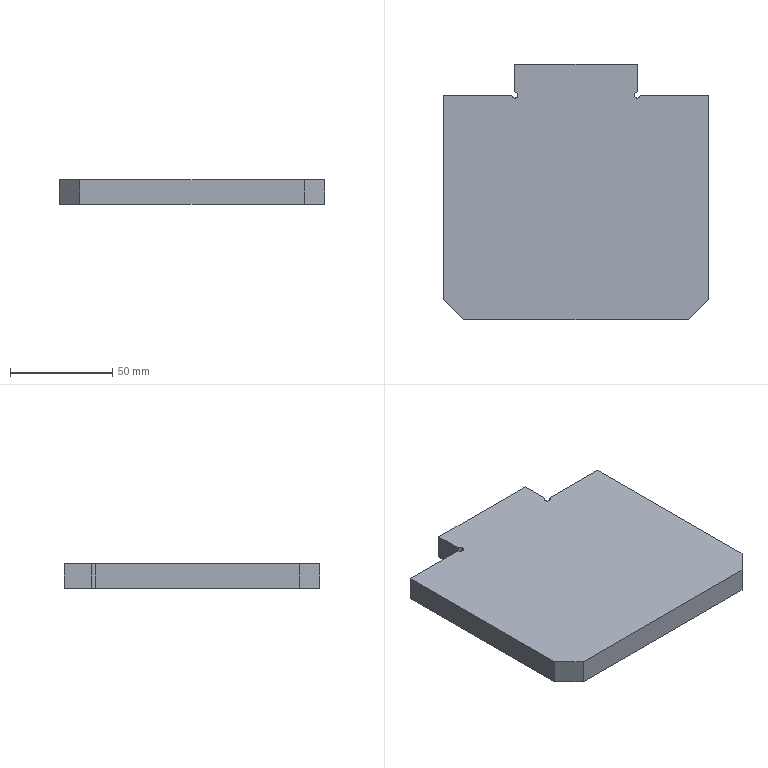Part | SolidWorks | features BaseBody 1 | 1 solid | 15 faces | box 130 x 125 x 12 mm | volume 181073 mm3 | plane 12 | cylinder 3 | commonest cylinder face diameters 3 x3
STEP:
#1=CARTESIAN_POINT('',(-28.5,55.,-6.));
#2=VERTEX_POINT('',#1);
#3=CARTESIAN_POINT('',(-30.,56.5,-6.));
#4=VERTEX_POINT('',#3);
#5=CARTESIAN_POINT('',(-30.,55.,-6.));
#6=DIRECTION('',(0.,0.,1.));
#7=DIRECTION('',(1.,0.,0.));
#8=AXIS2_PLACEMENT_3D('',#5,#6,#7);
#9=CIRCLE('',#8,1.5);
#10=EDGE_CURVE('',#2,#4,#9,.T.);
#11=ORIENTED_EDGE('',*,*,#10,.F.);
#12=CARTESIAN_POINT('',(-28.5,55.,6.));
#13=VERTEX_POINT('',#12);
#14=CARTESIAN_POINT('',(-28.5,55.,-7.));
#15=DIRECTION('',(0.,0.,1.));
#16=VECTOR('',#15,1000.);
#17=LINE('',#14,#16);
#18=EDGE_CURVE('',#2,#13,#17,.T.);
#19=ORIENTED_EDGE('',*,*,#18,.T.);
#20=CARTESIAN_POINT('',(-30.,56.5,6.));
#21=VERTEX_POINT('',#20);
#22=CARTESIAN_POINT('',(-30.,55.,6.));
#23=DIRECTION('',(0.,0.,1.));
#24=DIRECTION('',(1.,0.,0.));
#25=AXIS2_PLACEMENT_3D('',#22,#23,#24);
#26=CIRCLE('',#25,1.5);
#27=EDGE_CURVE('',#13,#21,#26,.T.);
#28=ORIENTED_EDGE('',*,*,#27,.T.);
#29=CARTESIAN_POINT('',(-30.,56.5,-7.));
#30=DIRECTION('',(0.,0.,1.));
#31=VECTOR('',#30,1000.);
#32=LINE('',#29,#31);
#33=EDGE_CURVE('',#4,#21,#32,.T.);
#34=ORIENTED_EDGE('',*,*,#33,.F.);
#35=EDGE_LOOP('',(#11,#19,#28,#34));
#36=FACE_OUTER_BOUND('',#35,.T.);
#37=CARTESIAN_POINT('',(-30.,55.,-7.));
#38=DIRECTION('',(0.,0.,1.));
#39=DIRECTION('',(1.,0.,0.));
#40=AXIS2_PLACEMENT_3D('',#37,#38,#39);
#41=CYLINDRICAL_SURFACE('',#40,1.5);
#42=ADVANCED_FACE('',(#36),#41,.F.);
#43=CARTESIAN_POINT('',(65.,55.,-6.));
#44=VERTEX_POINT('',#43);
#45=CARTESIAN_POINT('',(31.5,55.,-6.));
#46=VERTEX_POINT('',#45);
#47=CARTESIAN_POINT('',(-65.,55.,-6.));
#48=DIRECTION('',(-1.,0.,0.));
#49=VECTOR('',#48,1000.);
#50=LINE('',#47,#49);
#51=EDGE_CURVE('',#44,#46,#50,.T.);
#52=ORIENTED_EDGE('',*,*,#51,.T.);
#53=CARTESIAN_POINT('',(31.5,55.,6.));
#54=VERTEX_POINT('',#53);
#55=CARTESIAN_POINT('',(31.5,55.,-7.));
#56=DIRECTION('',(0.,0.,1.));
#57=VECTOR('',#56,1000.);
#58=LINE('',#55,#57);
#59=EDGE_CURVE('',#46,#54,#58,.T.);
#60=ORIENTED_EDGE('',*,*,#59,.T.);
#61=CARTESIAN_POINT('',(65.,55.,6.));
#62=VERTEX_POINT('',#61);
#63=CARTESIAN_POINT('',(-65.,55.,6.));
#64=DIRECTION('',(-1.,0.,0.));
#65=VECTOR('',#64,1000.);
#66=LINE('',#63,#65);
#67=EDGE_CURVE('',#62,#54,#66,.T.);
#68=ORIENTED_EDGE('',*,*,#67,.F.);
#69=CARTESIAN_POINT('',(65.,55.,6.));
#70=DIRECTION('',(0.,0.,-1.));
#71=VECTOR('',#70,1000.);
#72=LINE('',#69,#71);
#73=EDGE_CURVE('',#62,#44,#72,.T.);
#74=ORIENTED_EDGE('',*,*,#73,.T.);
#75=EDGE_LOOP('',(#52,#60,#68,#74));
#76=FACE_OUTER_BOUND('',#75,.T.);
#77=CARTESIAN_POINT('',(-65.,55.,6.));
#78=DIRECTION('',(0.,-1.,0.));
#79=DIRECTION('',(0.,0.,-1.));
#80=AXIS2_PLACEMENT_3D('',#77,#78,#79);
#81=PLANE('',#80);
#82=ADVANCED_FACE('',(#76),#81,.F.);
#83=CARTESIAN_POINT('',(65.,-45.,6.));
#84=VERTEX_POINT('',#83);
#85=CARTESIAN_POINT('',(65.,55.,6.));
#86=DIRECTION('',(0.,1.,0.));
#87=VECTOR('',#86,1000.);
#88=LINE('',#85,#87);
#89=EDGE_CURVE('',#84,#62,#88,.T.);
#90=ORIENTED_EDGE('',*,*,#89,.F.);
#91=CARTESIAN_POINT('',(65.,-45.,-6.));
#92=VERTEX_POINT('',#91);
#93=CARTESIAN_POINT('',(65.,-45.,6.));
#94=DIRECTION('',(0.,0.,-1.));
#95=VECTOR('',#94,1000.);
#96=LINE('',#93,#95);
#97=EDGE_CURVE('',#84,#92,#96,.T.);
#98=ORIENTED_EDGE('',*,*,#97,.T.);
#99=CARTESIAN_POINT('',(65.,55.,-6.));
#100=DIRECTION('',(0.,1.,0.));
#101=VECTOR('',#100,1000.);
#102=LINE('',#99,#101);
#103=EDGE_CURVE('',#92,#44,#102,.T.);
#104=ORIENTED_EDGE('',*,*,#103,.T.);
#105=ORIENTED_EDGE('',*,*,#73,.F.);
#106=EDGE_LOOP('',(#90,#98,#104,#105));
#107=FACE_OUTER_BOUND('',#106,.T.);
#108=CARTESIAN_POINT('',(65.,55.,6.));
#109=DIRECTION('',(-1.,0.,0.));
#110=DIRECTION('',(0.,0.,1.));
#111=AXIS2_PLACEMENT_3D('',#108,#109,#110);
#112=PLANE('',#111);
#113=ADVANCED_FACE('',(#107),#112,.F.);
#114=CARTESIAN_POINT('',(-31.5,55.,6.));
#115=VERTEX_POINT('',#114);
#116=CARTESIAN_POINT('',(-65.,55.,6.));
#117=VERTEX_POINT('',#116);
#118=CARTESIAN_POINT('',(-65.,55.,6.));
#119=DIRECTION('',(-1.,0.,0.));
#120=VECTOR('',#119,1000.);
#121=LINE('',#118,#120);
#122=EDGE_CURVE('',#115,#117,#121,.T.);
#123=ORIENTED_EDGE('',*,*,#122,.F.);
#124=CARTESIAN_POINT('',(-31.5,55.,-6.));
#125=VERTEX_POINT('',#124);
#126=CARTESIAN_POINT('',(-31.5,55.,-7.));
#127=DIRECTION('',(0.,0.,-1.));
#128=VECTOR('',#127,1000.);
#129=LINE('',#126,#128);
#130=EDGE_CURVE('',#115,#125,#129,.T.);
#131=ORIENTED_EDGE('',*,*,#130,.T.);
#132=CARTESIAN_POINT('',(-65.,55.,-6.));
#133=VERTEX_POINT('',#132);
#134=CARTESIAN_POINT('',(-65.,55.,-6.));
#135=DIRECTION('',(-1.,0.,0.));
#136=VECTOR('',#135,1000.);
#137=LINE('',#134,#136);
#138=EDGE_CURVE('',#125,#133,#137,.T.);
#139=ORIENTED_EDGE('',*,*,#138,.T.);
#140=CARTESIAN_POINT('',(-65.,55.,6.));
#141=DIRECTION('',(0.,0.,-1.));
#142=VECTOR('',#141,1000.);
#143=LINE('',#140,#142);
#144=EDGE_CURVE('',#117,#133,#143,.T.);
#145=ORIENTED_EDGE('',*,*,#144,.F.);
#146=EDGE_LOOP('',(#123,#131,#139,#145));
#147=FACE_OUTER_BOUND('',#146,.T.);
#148=CARTESIAN_POINT('',(-65.,55.,6.));
#149=DIRECTION('',(0.,-1.,0.));
#150=DIRECTION('',(0.,0.,-1.));
#151=AXIS2_PLACEMENT_3D('',#148,#149,#150);
#152=PLANE('',#151);
#153=ADVANCED_FACE('',(#147),#152,.F.);
#154=CARTESIAN_POINT('',(-65.,-45.,-6.));
#155=VERTEX_POINT('',#154);
#156=CARTESIAN_POINT('',(-65.,55.,-6.));
#157=DIRECTION('',(0.,-1.,0.));
#158=VECTOR('',#157,1000.);
#159=LINE('',#156,#158);
#160=EDGE_CURVE('',#133,#155,#159,.T.);
#161=ORIENTED_EDGE('',*,*,#160,.T.);
#162=CARTESIAN_POINT('',(-65.,-45.,6.));
#163=VERTEX_POINT('',#162);
#164=CARTESIAN_POINT('',(-65.,-45.,6.));
#165=DIRECTION('',(0.,0.,1.));
#166=VECTOR('',#165,1000.);
#167=LINE('',#164,#166);
#168=EDGE_CURVE('',#155,#163,#167,.T.);
#169=ORIENTED_EDGE('',*,*,#168,.T.);
#170=CARTESIAN_POINT('',(-65.,55.,6.));
#171=DIRECTION('',(0.,-1.,0.));
#172=VECTOR('',#171,1000.);
#173=LINE('',#170,#172);
#174=EDGE_CURVE('',#117,#163,#173,.T.);
#175=ORIENTED_EDGE('',*,*,#174,.F.);
#176=ORIENTED_EDGE('',*,*,#144,.T.);
#177=EDGE_LOOP('',(#161,#169,#175,#176));
#178=FACE_OUTER_BOUND('',#177,.T.);
#179=CARTESIAN_POINT('',(-65.,55.,6.));
#180=DIRECTION('',(1.,0.,0.));
#181=DIRECTION('',(0.,0.,-1.));
#182=AXIS2_PLACEMENT_3D('',#179,#180,#181);
#183=PLANE('',#182);
#184=ADVANCED_FACE('',(#178),#183,.F.);
#185=CARTESIAN_POINT('',(-55.,-55.,-6.));
#186=VERTEX_POINT('',#185);
#187=CARTESIAN_POINT('',(55.,-55.,-6.));
#188=VERTEX_POINT('',#187);
#189=CARTESIAN_POINT('',(-65.,-55.,-6.));
#190=DIRECTION('',(1.,0.,0.));
#191=VECTOR('',#190,1000.);
#192=LINE('',#189,#191);
#193=EDGE_CURVE('',#186,#188,#192,.T.);
#194=ORIENTED_EDGE('',*,*,#193,.T.);
#195=CARTESIAN_POINT('',(55.,-55.,6.));
#196=VERTEX_POINT('',#195);
#197=CARTESIAN_POINT('',(55.,-55.,6.));
#198=DIRECTION('',(0.,0.,1.));
#199=VECTOR('',#198,1000.);
#200=LINE('',#197,#199);
#201=EDGE_CURVE('',#188,#196,#200,.T.);
#202=ORIENTED_EDGE('',*,*,#201,.T.);
#203=CARTESIAN_POINT('',(-55.,-55.,6.));
#204=VERTEX_POINT('',#203);
#205=CARTESIAN_POINT('',(-65.,-55.,6.));
#206=DIRECTION('',(1.,0.,0.));
#207=VECTOR('',#206,1000.);
#208=LINE('',#205,#207);
#209=EDGE_CURVE('',#204,#196,#208,.T.);
#210=ORIENTED_EDGE('',*,*,#209,.F.);
#211=CARTESIAN_POINT('',(-55.,-55.,6.));
#212=DIRECTION('',(0.,0.,-1.));
#213=VECTOR('',#212,1000.);
#214=LINE('',#211,#213);
#215=EDGE_CURVE('',#204,#186,#214,.T.);
#216=ORIENTED_EDGE('',*,*,#215,.T.);
#217=EDGE_LOOP('',(#194,#202,#210,#216));
#218=FACE_OUTER_BOUND('',#217,.T.);
#219=CARTESIAN_POINT('',(-65.,-55.,6.));
#220=DIRECTION('',(0.,1.,0.));
#221=DIRECTION('',(0.,0.,1.));
#222=AXIS2_PLACEMENT_3D('',#219,#220,#221);
#223=PLANE('',#222);
#224=ADVANCED_FACE('',(#218),#223,.F.);
#225=CARTESIAN_POINT('',(-30.,55.,6.));
#226=DIRECTION('',(0.,0.,1.));
#227=DIRECTION('',(1.,0.,0.));
#228=AXIS2_PLACEMENT_3D('',#225,#226,#227);
#229=CIRCLE('',#228,1.5);
#230=EDGE_CURVE('',#115,#13,#229,.T.);
#231=ORIENTED_EDGE('',*,*,#230,.F.);
#232=ORIENTED_EDGE('',*,*,#122,.T.);
#233=ORIENTED_EDGE('',*,*,#174,.T.);
#234=CARTESIAN_POINT('',(-55.,-55.,6.));
#235=DIRECTION('',(0.7071,-0.7071,0.));
#236=VECTOR('',#235,1000.);
#237=LINE('',#234,#236);
#238=EDGE_CURVE('',#163,#204,#237,.T.);
#239=ORIENTED_EDGE('',*,*,#238,.T.);
#240=ORIENTED_EDGE('',*,*,#209,.T.);
#241=CARTESIAN_POINT('',(55.,-55.,6.));
#242=DIRECTION('',(0.7071,0.7071,0.));
#243=VECTOR('',#242,1000.);
#244=LINE('',#241,#243);
#245=EDGE_CURVE('',#196,#84,#244,.T.);
#246=ORIENTED_EDGE('',*,*,#245,.T.);
#247=ORIENTED_EDGE('',*,*,#89,.T.);
#248=ORIENTED_EDGE('',*,*,#67,.T.);
#249=CARTESIAN_POINT('',(30.,56.5,6.));
#250=VERTEX_POINT('',#249);
#251=CARTESIAN_POINT('',(30.,55.,6.));
#252=DIRECTION('',(0.,0.,1.));
#253=DIRECTION('',(1.,0.,0.));
#254=AXIS2_PLACEMENT_3D('',#251,#252,#253);
#255=CIRCLE('',#254,1.5);
#256=EDGE_CURVE('',#250,#54,#255,.T.);
#257=ORIENTED_EDGE('',*,*,#256,.F.);
#258=CARTESIAN_POINT('',(30.,70.,6.));
#259=VERTEX_POINT('',#258);
#260=CARTESIAN_POINT('',(30.,55.,6.));
#261=DIRECTION('',(0.,1.,0.));
#262=VECTOR('',#261,1000.);
#263=LINE('',#260,#262);
#264=EDGE_CURVE('',#250,#259,#263,.T.);
#265=ORIENTED_EDGE('',*,*,#264,.T.);
#266=CARTESIAN_POINT('',(-30.,70.,6.));
#267=VERTEX_POINT('',#266);
#268=CARTESIAN_POINT('',(-30.,70.,6.));
#269=DIRECTION('',(-1.,0.,0.));
#270=VECTOR('',#269,1000.);
#271=LINE('',#268,#270);
#272=EDGE_CURVE('',#259,#267,#271,.T.);
#273=ORIENTED_EDGE('',*,*,#272,.T.);
#274=CARTESIAN_POINT('',(-30.,55.,6.));
#275=DIRECTION('',(0.,-1.,0.));
#276=VECTOR('',#275,1000.);
#277=LINE('',#274,#276);
#278=EDGE_CURVE('',#267,#21,#277,.T.);
#279=ORIENTED_EDGE('',*,*,#278,.T.);
#280=ORIENTED_EDGE('',*,*,#27,.F.);
#281=EDGE_LOOP('',(#231,#232,#233,#239,#240,#246,#247,#248,#257,#265,#273,#279,#280));
#282=FACE_OUTER_BOUND('',#281,.T.);
#283=CARTESIAN_POINT('',(0.,0.,6.));
#284=DIRECTION('',(0.,0.,1.));
#285=DIRECTION('',(1.,0.,0.));
#286=AXIS2_PLACEMENT_3D('',#283,#284,#285);
#287=PLANE('',#286);
#288=ADVANCED_FACE('',(#282),#287,.T.);
#289=ORIENTED_EDGE('',*,*,#138,.F.);
#290=CARTESIAN_POINT('',(-30.,55.,-6.));
#291=DIRECTION('',(0.,0.,1.));
#292=DIRECTION('',(1.,0.,0.));
#293=AXIS2_PLACEMENT_3D('',#290,#291,#292);
#294=CIRCLE('',#293,1.5);
#295=EDGE_CURVE('',#125,#2,#294,.T.);
#296=ORIENTED_EDGE('',*,*,#295,.T.);
#297=ORIENTED_EDGE('',*,*,#10,.T.);
#298=CARTESIAN_POINT('',(-30.,70.,-6.));
#299=VERTEX_POINT('',#298);
#300=CARTESIAN_POINT('',(-30.,55.,-6.));
#301=DIRECTION('',(0.,-1.,0.));
#302=VECTOR('',#301,1000.);
#303=LINE('',#300,#302);
#304=EDGE_CURVE('',#299,#4,#303,.T.);
#305=ORIENTED_EDGE('',*,*,#304,.F.);
#306=CARTESIAN_POINT('',(30.,70.,-6.));
#307=VERTEX_POINT('',#306);
#308=CARTESIAN_POINT('',(-30.,70.,-6.));
#309=DIRECTION('',(-1.,0.,0.));
#310=VECTOR('',#309,1000.);
#311=LINE('',#308,#310);
#312=EDGE_CURVE('',#307,#299,#311,.T.);
#313=ORIENTED_EDGE('',*,*,#312,.F.);
#314=CARTESIAN_POINT('',(30.,56.5,-6.));
#315=VERTEX_POINT('',#314);
#316=CARTESIAN_POINT('',(30.,55.,-6.));
#317=DIRECTION('',(0.,1.,0.));
#318=VECTOR('',#317,1000.);
#319=LINE('',#316,#318);
#320=EDGE_CURVE('',#315,#307,#319,.T.);
#321=ORIENTED_EDGE('',*,*,#320,.F.);
#322=CARTESIAN_POINT('',(30.,55.,-6.));
#323=DIRECTION('',(0.,0.,1.));
#324=DIRECTION('',(1.,0.,0.));
#325=AXIS2_PLACEMENT_3D('',#322,#323,#324);
#326=CIRCLE('',#325,1.5);
#327=EDGE_CURVE('',#315,#46,#326,.T.);
#328=ORIENTED_EDGE('',*,*,#327,.T.);
#329=ORIENTED_EDGE('',*,*,#51,.F.);
#330=ORIENTED_EDGE('',*,*,#103,.F.);
#331=CARTESIAN_POINT('',(65.,-45.,-6.));
#332=DIRECTION('',(-0.7071,-0.7071,0.));
#333=VECTOR('',#332,1000.);
#334=LINE('',#331,#333);
#335=EDGE_CURVE('',#92,#188,#334,.T.);
#336=ORIENTED_EDGE('',*,*,#335,.T.);
#337=ORIENTED_EDGE('',*,*,#193,.F.);
#338=CARTESIAN_POINT('',(-55.,-55.,-6.));
#339=DIRECTION('',(-0.7071,0.7071,0.));
#340=VECTOR('',#339,1000.);
#341=LINE('',#338,#340);
#342=EDGE_CURVE('',#186,#155,#341,.T.);
#343=ORIENTED_EDGE('',*,*,#342,.T.);
#344=ORIENTED_EDGE('',*,*,#160,.F.);
#345=EDGE_LOOP('',(#289,#296,#297,#305,#313,#321,#328,#329,#330,#336,#337,#343,#344));
#346=FACE_OUTER_BOUND('',#345,.T.);
#347=CARTESIAN_POINT('',(0.,0.,-6.));
#348=DIRECTION('',(0.,0.,1.));
#349=DIRECTION('',(1.,0.,0.));
#350=AXIS2_PLACEMENT_3D('',#347,#348,#349);
#351=PLANE('',#350);
#352=ADVANCED_FACE('',(#346),#351,.F.);
#353=ORIENTED_EDGE('',*,*,#304,.T.);
#354=ORIENTED_EDGE('',*,*,#33,.T.);
#355=ORIENTED_EDGE('',*,*,#278,.F.);
#356=CARTESIAN_POINT('',(-30.,70.,6.));
#357=DIRECTION('',(0.,0.,-1.));
#358=VECTOR('',#357,1000.);
#359=LINE('',#356,#358);
#360=EDGE_CURVE('',#267,#299,#359,.T.);
#361=ORIENTED_EDGE('',*,*,#360,.T.);
#362=EDGE_LOOP('',(#353,#354,#355,#361));
#363=FACE_OUTER_BOUND('',#362,.T.);
#364=CARTESIAN_POINT('',(-30.,55.,6.));
#365=DIRECTION('',(1.,0.,0.));
#366=DIRECTION('',(0.,0.,-1.));
#367=AXIS2_PLACEMENT_3D('',#364,#365,#366);
#368=PLANE('',#367);
#369=ADVANCED_FACE('',(#363),#368,.F.);
#370=ORIENTED_EDGE('',*,*,#264,.F.);
#371=CARTESIAN_POINT('',(30.,56.5,-7.));
#372=DIRECTION('',(0.,0.,-1.));
#373=VECTOR('',#372,1000.);
#374=LINE('',#371,#373);
#375=EDGE_CURVE('',#250,#315,#374,.T.);
#376=ORIENTED_EDGE('',*,*,#375,.T.);
#377=ORIENTED_EDGE('',*,*,#320,.T.);
#378=CARTESIAN_POINT('',(30.,70.,6.));
#379=DIRECTION('',(0.,0.,-1.));
#380=VECTOR('',#379,1000.);
#381=LINE('',#378,#380);
#382=EDGE_CURVE('',#259,#307,#381,.T.);
#383=ORIENTED_EDGE('',*,*,#382,.F.);
#384=EDGE_LOOP('',(#370,#376,#377,#383));
#385=FACE_OUTER_BOUND('',#384,.T.);
#386=CARTESIAN_POINT('',(30.,55.,6.));
#387=DIRECTION('',(-1.,0.,0.));
#388=DIRECTION('',(0.,0.,1.));
#389=AXIS2_PLACEMENT_3D('',#386,#387,#388);
#390=PLANE('',#389);
#391=ADVANCED_FACE('',(#385),#390,.F.);
#392=ORIENTED_EDGE('',*,*,#312,.T.);
#393=ORIENTED_EDGE('',*,*,#360,.F.);
#394=ORIENTED_EDGE('',*,*,#272,.F.);
#395=ORIENTED_EDGE('',*,*,#382,.T.);
#396=EDGE_LOOP('',(#392,#393,#394,#395));
#397=FACE_OUTER_BOUND('',#396,.T.);
#398=CARTESIAN_POINT('',(-30.,70.,6.));
#399=DIRECTION('',(0.,-1.,0.));
#400=DIRECTION('',(0.,0.,-1.));
#401=AXIS2_PLACEMENT_3D('',#398,#399,#400);
#402=PLANE('',#401);
#403=ADVANCED_FACE('',(#397),#402,.F.);
#404=ORIENTED_EDGE('',*,*,#245,.F.);
#405=ORIENTED_EDGE('',*,*,#201,.F.);
#406=ORIENTED_EDGE('',*,*,#335,.F.);
#407=ORIENTED_EDGE('',*,*,#97,.F.);
#408=EDGE_LOOP('',(#404,#405,#406,#407));
#409=FACE_OUTER_BOUND('',#408,.T.);
#410=CARTESIAN_POINT('',(65.,-45.,6.));
#411=DIRECTION('',(-0.7071,0.7071,0.));
#412=DIRECTION('',(0.,0.,-1.));
#413=AXIS2_PLACEMENT_3D('',#410,#411,#412);
#414=PLANE('',#413);
#415=ADVANCED_FACE('',(#409),#414,.F.);
#416=ORIENTED_EDGE('',*,*,#238,.F.);
#417=ORIENTED_EDGE('',*,*,#168,.F.);
#418=ORIENTED_EDGE('',*,*,#342,.F.);
#419=ORIENTED_EDGE('',*,*,#215,.F.);
#420=EDGE_LOOP('',(#416,#417,#418,#419));
#421=FACE_OUTER_BOUND('',#420,.T.);
#422=CARTESIAN_POINT('',(-55.,-55.,6.));
#423=DIRECTION('',(0.7071,0.7071,0.));
#424=DIRECTION('',(0.,0.,-1.));
#425=AXIS2_PLACEMENT_3D('',#422,#423,#424);
#426=PLANE('',#425);
#427=ADVANCED_FACE('',(#421),#426,.F.);
#428=ORIENTED_EDGE('',*,*,#327,.F.);
#429=ORIENTED_EDGE('',*,*,#375,.F.);
#430=ORIENTED_EDGE('',*,*,#256,.T.);
#431=ORIENTED_EDGE('',*,*,#59,.F.);
#432=EDGE_LOOP('',(#428,#429,#430,#431));
#433=FACE_OUTER_BOUND('',#432,.T.);
#434=CARTESIAN_POINT('',(30.,55.,-7.));
#435=DIRECTION('',(0.,0.,1.));
#436=DIRECTION('',(1.,0.,0.));
#437=AXIS2_PLACEMENT_3D('',#434,#435,#436);
#438=CYLINDRICAL_SURFACE('',#437,1.5);
#439=ADVANCED_FACE('',(#433),#438,.F.);
#440=ORIENTED_EDGE('',*,*,#18,.F.);
#441=ORIENTED_EDGE('',*,*,#295,.F.);
#442=ORIENTED_EDGE('',*,*,#130,.F.);
#443=ORIENTED_EDGE('',*,*,#230,.T.);
#444=EDGE_LOOP('',(#440,#441,#442,#443));
#445=FACE_OUTER_BOUND('',#444,.T.);
#446=CARTESIAN_POINT('',(-30.,55.,-7.));
#447=DIRECTION('',(0.,0.,1.));
#448=DIRECTION('',(1.,0.,0.));
#449=AXIS2_PLACEMENT_3D('',#446,#447,#448);
#450=CYLINDRICAL_SURFACE('',#449,1.5);
#451=ADVANCED_FACE('',(#445),#450,.F.);
#452=CLOSED_SHELL('',(#42,#82,#113,#153,#184,#224,#288,#352,#369,#391,#403,#415,#427,#439,#451));
#453=MANIFOLD_SOLID_BREP('',#452);
#454=CARTESIAN_POINT('',(0.,0.,0.));
#455=DIRECTION('',(0.,0.,1.));
#456=DIRECTION('',(1.,0.,0.));
#457=AXIS2_PLACEMENT_3D('',#454,#455,#456);
#458=(LENGTH_UNIT()NAMED_UNIT(*)SI_UNIT(.MILLI.,.METRE.));
#459=UNCERTAINTY_MEASURE_WITH_UNIT(LENGTH_MEASURE(0.00001),#458,'','');
#460=(NAMED_UNIT(*)PLANE_ANGLE_UNIT()SI_UNIT($,.RADIAN.));
#461=(NAMED_UNIT(*)SI_UNIT($,.STERADIAN.)SOLID_ANGLE_UNIT());
#462=(GEOMETRIC_REPRESENTATION_CONTEXT(3)GLOBAL_UNCERTAINTY_ASSIGNED_CONTEXT((#459))GLOBAL_UNIT_ASSIGNED_CONTEXT((#458,#460,#461))REPRESENTATION_CONTEXT('',''));
#463=ADVANCED_BREP_SHAPE_REPRESENTATION('',(#453,#457),#462);